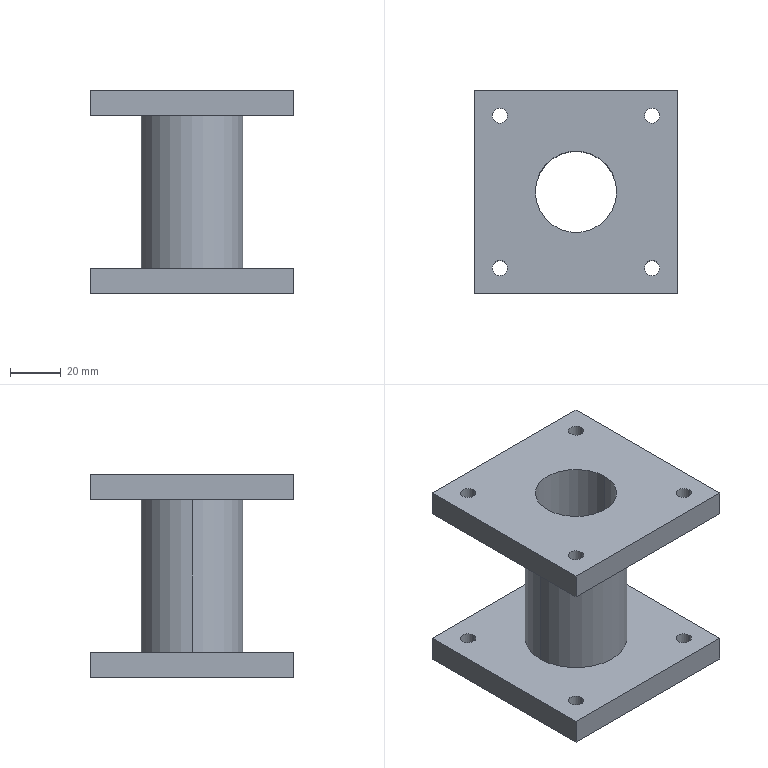Part | STEP file | Square tube | 1 solid | 32 faces | box 80 x 80 x 80 mm | volume 136796 mm3 | cylinder 20 | plane 12 | commonest cylinder face diameters 6 x16 32 x2 40 x2
STEP:
#1=CARTESIAN_POINT('',(33.,-30.,10.));
#2=VERTEX_POINT('',#1);
#3=CARTESIAN_POINT('',(27.,-30.,10.));
#4=VERTEX_POINT('',#3);
#5=CARTESIAN_POINT('',(30.,-30.,10.));
#6=DIRECTION('',(0.,0.,-1.));
#7=DIRECTION('',(-1.,0.,0.));
#8=AXIS2_PLACEMENT_3D('',#5,#6,#7);
#9=CIRCLE('',#8,3.);
#10=EDGE_CURVE('',#2,#4,#9,.T.);
#11=ORIENTED_EDGE('',*,*,#10,.F.);
#12=CARTESIAN_POINT('',(33.,-30.,0.));
#13=VERTEX_POINT('',#12);
#14=CARTESIAN_POINT('',(33.,-30.,10.));
#15=DIRECTION('',(0.,0.,-1.));
#16=VECTOR('',#15,1000.);
#17=LINE('',#14,#16);
#18=EDGE_CURVE('',#2,#13,#17,.T.);
#19=ORIENTED_EDGE('',*,*,#18,.T.);
#20=CARTESIAN_POINT('',(27.,-30.,0.));
#21=VERTEX_POINT('',#20);
#22=CARTESIAN_POINT('',(30.,-30.,0.));
#23=DIRECTION('',(0.,0.,-1.));
#24=DIRECTION('',(-1.,0.,0.));
#25=AXIS2_PLACEMENT_3D('',#22,#23,#24);
#26=CIRCLE('',#25,3.);
#27=EDGE_CURVE('',#13,#21,#26,.T.);
#28=ORIENTED_EDGE('',*,*,#27,.T.);
#29=CARTESIAN_POINT('',(27.,-30.,10.));
#30=DIRECTION('',(0.,0.,-1.));
#31=VECTOR('',#30,1000.);
#32=LINE('',#29,#31);
#33=EDGE_CURVE('',#4,#21,#32,.T.);
#34=ORIENTED_EDGE('',*,*,#33,.F.);
#35=EDGE_LOOP('',(#11,#19,#28,#34));
#36=FACE_OUTER_BOUND('',#35,.T.);
#37=CARTESIAN_POINT('',(30.,-30.,10.));
#38=DIRECTION('',(0.,0.,-1.));
#39=DIRECTION('',(-1.,0.,0.));
#40=AXIS2_PLACEMENT_3D('',#37,#38,#39);
#41=CYLINDRICAL_SURFACE('',#40,3.);
#42=ADVANCED_FACE('',(#36),#41,.F.);
#43=CARTESIAN_POINT('',(33.,30.,10.));
#44=VERTEX_POINT('',#43);
#45=CARTESIAN_POINT('',(27.,30.,10.));
#46=VERTEX_POINT('',#45);
#47=CARTESIAN_POINT('',(30.,30.,10.));
#48=DIRECTION('',(0.,0.,-1.));
#49=DIRECTION('',(-1.,0.,0.));
#50=AXIS2_PLACEMENT_3D('',#47,#48,#49);
#51=CIRCLE('',#50,3.);
#52=EDGE_CURVE('',#44,#46,#51,.T.);
#53=ORIENTED_EDGE('',*,*,#52,.F.);
#54=CARTESIAN_POINT('',(33.,30.,0.));
#55=VERTEX_POINT('',#54);
#56=CARTESIAN_POINT('',(33.,30.,10.));
#57=DIRECTION('',(0.,0.,-1.));
#58=VECTOR('',#57,1000.);
#59=LINE('',#56,#58);
#60=EDGE_CURVE('',#44,#55,#59,.T.);
#61=ORIENTED_EDGE('',*,*,#60,.T.);
#62=CARTESIAN_POINT('',(27.,30.,0.));
#63=VERTEX_POINT('',#62);
#64=CARTESIAN_POINT('',(30.,30.,0.));
#65=DIRECTION('',(0.,0.,-1.));
#66=DIRECTION('',(-1.,0.,0.));
#67=AXIS2_PLACEMENT_3D('',#64,#65,#66);
#68=CIRCLE('',#67,3.);
#69=EDGE_CURVE('',#55,#63,#68,.T.);
#70=ORIENTED_EDGE('',*,*,#69,.T.);
#71=CARTESIAN_POINT('',(27.,30.,10.));
#72=DIRECTION('',(0.,0.,-1.));
#73=VECTOR('',#72,1000.);
#74=LINE('',#71,#73);
#75=EDGE_CURVE('',#46,#63,#74,.T.);
#76=ORIENTED_EDGE('',*,*,#75,.F.);
#77=EDGE_LOOP('',(#53,#61,#70,#76));
#78=FACE_OUTER_BOUND('',#77,.T.);
#79=CARTESIAN_POINT('',(30.,30.,10.));
#80=DIRECTION('',(0.,0.,-1.));
#81=DIRECTION('',(-1.,0.,0.));
#82=AXIS2_PLACEMENT_3D('',#79,#80,#81);
#83=CYLINDRICAL_SURFACE('',#82,3.);
#84=ADVANCED_FACE('',(#78),#83,.F.);
#85=CARTESIAN_POINT('',(-27.,30.,10.));
#86=VERTEX_POINT('',#85);
#87=CARTESIAN_POINT('',(-33.,30.,10.));
#88=VERTEX_POINT('',#87);
#89=CARTESIAN_POINT('',(-30.,30.,10.));
#90=DIRECTION('',(0.,0.,-1.));
#91=DIRECTION('',(-1.,0.,0.));
#92=AXIS2_PLACEMENT_3D('',#89,#90,#91);
#93=CIRCLE('',#92,3.);
#94=EDGE_CURVE('',#86,#88,#93,.T.);
#95=ORIENTED_EDGE('',*,*,#94,.F.);
#96=CARTESIAN_POINT('',(-27.,30.,0.));
#97=VERTEX_POINT('',#96);
#98=CARTESIAN_POINT('',(-27.,30.,10.));
#99=DIRECTION('',(0.,0.,-1.));
#100=VECTOR('',#99,1000.);
#101=LINE('',#98,#100);
#102=EDGE_CURVE('',#86,#97,#101,.T.);
#103=ORIENTED_EDGE('',*,*,#102,.T.);
#104=CARTESIAN_POINT('',(-33.,30.,0.));
#105=VERTEX_POINT('',#104);
#106=CARTESIAN_POINT('',(-30.,30.,0.));
#107=DIRECTION('',(0.,0.,-1.));
#108=DIRECTION('',(-1.,0.,0.));
#109=AXIS2_PLACEMENT_3D('',#106,#107,#108);
#110=CIRCLE('',#109,3.);
#111=EDGE_CURVE('',#97,#105,#110,.T.);
#112=ORIENTED_EDGE('',*,*,#111,.T.);
#113=CARTESIAN_POINT('',(-33.,30.,10.));
#114=DIRECTION('',(0.,0.,-1.));
#115=VECTOR('',#114,1000.);
#116=LINE('',#113,#115);
#117=EDGE_CURVE('',#88,#105,#116,.T.);
#118=ORIENTED_EDGE('',*,*,#117,.F.);
#119=EDGE_LOOP('',(#95,#103,#112,#118));
#120=FACE_OUTER_BOUND('',#119,.T.);
#121=CARTESIAN_POINT('',(-30.,30.,10.));
#122=DIRECTION('',(0.,0.,-1.));
#123=DIRECTION('',(-1.,0.,0.));
#124=AXIS2_PLACEMENT_3D('',#121,#122,#123);
#125=CYLINDRICAL_SURFACE('',#124,3.);
#126=ADVANCED_FACE('',(#120),#125,.F.);
#127=CARTESIAN_POINT('',(-27.,-30.,10.));
#128=VERTEX_POINT('',#127);
#129=CARTESIAN_POINT('',(-33.,-30.,10.));
#130=VERTEX_POINT('',#129);
#131=CARTESIAN_POINT('',(-30.,-30.,10.));
#132=DIRECTION('',(0.,0.,-1.));
#133=DIRECTION('',(-1.,0.,0.));
#134=AXIS2_PLACEMENT_3D('',#131,#132,#133);
#135=CIRCLE('',#134,3.);
#136=EDGE_CURVE('',#128,#130,#135,.T.);
#137=ORIENTED_EDGE('',*,*,#136,.F.);
#138=CARTESIAN_POINT('',(-27.,-30.,0.));
#139=VERTEX_POINT('',#138);
#140=CARTESIAN_POINT('',(-27.,-30.,10.));
#141=DIRECTION('',(0.,0.,-1.));
#142=VECTOR('',#141,1000.);
#143=LINE('',#140,#142);
#144=EDGE_CURVE('',#128,#139,#143,.T.);
#145=ORIENTED_EDGE('',*,*,#144,.T.);
#146=CARTESIAN_POINT('',(-33.,-30.,0.));
#147=VERTEX_POINT('',#146);
#148=CARTESIAN_POINT('',(-30.,-30.,0.));
#149=DIRECTION('',(0.,0.,-1.));
#150=DIRECTION('',(-1.,0.,0.));
#151=AXIS2_PLACEMENT_3D('',#148,#149,#150);
#152=CIRCLE('',#151,3.);
#153=EDGE_CURVE('',#139,#147,#152,.T.);
#154=ORIENTED_EDGE('',*,*,#153,.T.);
#155=CARTESIAN_POINT('',(-33.,-30.,10.));
#156=DIRECTION('',(0.,0.,-1.));
#157=VECTOR('',#156,1000.);
#158=LINE('',#155,#157);
#159=EDGE_CURVE('',#130,#147,#158,.T.);
#160=ORIENTED_EDGE('',*,*,#159,.F.);
#161=EDGE_LOOP('',(#137,#145,#154,#160));
#162=FACE_OUTER_BOUND('',#161,.T.);
#163=CARTESIAN_POINT('',(-30.,-30.,10.));
#164=DIRECTION('',(0.,0.,-1.));
#165=DIRECTION('',(-1.,0.,0.));
#166=AXIS2_PLACEMENT_3D('',#163,#164,#165);
#167=CYLINDRICAL_SURFACE('',#166,3.);
#168=ADVANCED_FACE('',(#162),#167,.F.);
#169=CARTESIAN_POINT('',(16.,0.,80.));
#170=VERTEX_POINT('',#169);
#171=CARTESIAN_POINT('',(-16.,0.,80.));
#172=VERTEX_POINT('',#171);
#173=CARTESIAN_POINT('',(0.,0.,80.));
#174=DIRECTION('',(0.,0.,-1.));
#175=DIRECTION('',(-1.,0.,0.));
#176=AXIS2_PLACEMENT_3D('',#173,#174,#175);
#177=CIRCLE('',#176,16.);
#178=EDGE_CURVE('',#170,#172,#177,.T.);
#179=ORIENTED_EDGE('',*,*,#178,.F.);
#180=CARTESIAN_POINT('',(16.,0.,0.));
#181=VERTEX_POINT('',#180);
#182=CARTESIAN_POINT('',(16.,0.,70.));
#183=DIRECTION('',(0.,0.,-1.));
#184=VECTOR('',#183,1000.);
#185=LINE('',#182,#184);
#186=EDGE_CURVE('',#170,#181,#185,.T.);
#187=ORIENTED_EDGE('',*,*,#186,.T.);
#188=CARTESIAN_POINT('',(-16.,0.,0.));
#189=VERTEX_POINT('',#188);
#190=CARTESIAN_POINT('',(0.,0.,0.));
#191=DIRECTION('',(0.,0.,-1.));
#192=DIRECTION('',(-1.,0.,0.));
#193=AXIS2_PLACEMENT_3D('',#190,#191,#192);
#194=CIRCLE('',#193,16.);
#195=EDGE_CURVE('',#181,#189,#194,.T.);
#196=ORIENTED_EDGE('',*,*,#195,.T.);
#197=CARTESIAN_POINT('',(-16.,0.,70.));
#198=DIRECTION('',(0.,0.,-1.));
#199=VECTOR('',#198,1000.);
#200=LINE('',#197,#199);
#201=EDGE_CURVE('',#172,#189,#200,.T.);
#202=ORIENTED_EDGE('',*,*,#201,.F.);
#203=EDGE_LOOP('',(#179,#187,#196,#202));
#204=FACE_OUTER_BOUND('',#203,.T.);
#205=CARTESIAN_POINT('',(0.,0.,70.));
#206=DIRECTION('',(0.,0.,-1.));
#207=DIRECTION('',(-1.,0.,0.));
#208=AXIS2_PLACEMENT_3D('',#205,#206,#207);
#209=CYLINDRICAL_SURFACE('',#208,16.);
#210=ADVANCED_FACE('',(#204),#209,.F.);
#211=CARTESIAN_POINT('',(-20.,0.,70.));
#212=VERTEX_POINT('',#211);
#213=CARTESIAN_POINT('',(20.,0.,70.));
#214=VERTEX_POINT('',#213);
#215=CARTESIAN_POINT('',(0.,0.,70.));
#216=DIRECTION('',(0.,0.,-1.));
#217=DIRECTION('',(-1.,0.,0.));
#218=AXIS2_PLACEMENT_3D('',#215,#216,#217);
#219=CIRCLE('',#218,20.);
#220=EDGE_CURVE('',#212,#214,#219,.T.);
#221=ORIENTED_EDGE('',*,*,#220,.T.);
#222=CARTESIAN_POINT('',(20.,0.,10.));
#223=VERTEX_POINT('',#222);
#224=CARTESIAN_POINT('',(20.,0.,70.));
#225=DIRECTION('',(0.,0.,-1.));
#226=VECTOR('',#225,1000.);
#227=LINE('',#224,#226);
#228=EDGE_CURVE('',#214,#223,#227,.T.);
#229=ORIENTED_EDGE('',*,*,#228,.T.);
#230=CARTESIAN_POINT('',(-20.,0.,10.));
#231=VERTEX_POINT('',#230);
#232=CARTESIAN_POINT('',(0.,0.,10.));
#233=DIRECTION('',(0.,0.,-1.));
#234=DIRECTION('',(-1.,0.,0.));
#235=AXIS2_PLACEMENT_3D('',#232,#233,#234);
#236=CIRCLE('',#235,20.);
#237=EDGE_CURVE('',#231,#223,#236,.T.);
#238=ORIENTED_EDGE('',*,*,#237,.F.);
#239=CARTESIAN_POINT('',(-20.,0.,70.));
#240=DIRECTION('',(0.,0.,-1.));
#241=VECTOR('',#240,1000.);
#242=LINE('',#239,#241);
#243=EDGE_CURVE('',#212,#231,#242,.T.);
#244=ORIENTED_EDGE('',*,*,#243,.F.);
#245=EDGE_LOOP('',(#221,#229,#238,#244));
#246=FACE_OUTER_BOUND('',#245,.T.);
#247=CARTESIAN_POINT('',(0.,0.,70.));
#248=DIRECTION('',(0.,0.,-1.));
#249=DIRECTION('',(-1.,0.,0.));
#250=AXIS2_PLACEMENT_3D('',#247,#248,#249);
#251=CYLINDRICAL_SURFACE('',#250,20.);
#252=ADVANCED_FACE('',(#246),#251,.T.);
#253=CARTESIAN_POINT('',(-27.,-30.,80.));
#254=VERTEX_POINT('',#253);
#255=CARTESIAN_POINT('',(-33.,-30.,80.));
#256=VERTEX_POINT('',#255);
#257=CARTESIAN_POINT('',(-30.,-30.,80.));
#258=DIRECTION('',(0.,0.,-1.));
#259=DIRECTION('',(-1.,0.,0.));
#260=AXIS2_PLACEMENT_3D('',#257,#258,#259);
#261=CIRCLE('',#260,3.);
#262=EDGE_CURVE('',#254,#256,#261,.T.);
#263=ORIENTED_EDGE('',*,*,#262,.F.);
#264=CARTESIAN_POINT('',(-27.,-30.,70.));
#265=VERTEX_POINT('',#264);
#266=CARTESIAN_POINT('',(-27.,-30.,80.));
#267=DIRECTION('',(0.,0.,-1.));
#268=VECTOR('',#267,1000.);
#269=LINE('',#266,#268);
#270=EDGE_CURVE('',#254,#265,#269,.T.);
#271=ORIENTED_EDGE('',*,*,#270,.T.);
#272=CARTESIAN_POINT('',(-33.,-30.,70.));
#273=VERTEX_POINT('',#272);
#274=CARTESIAN_POINT('',(-30.,-30.,70.));
#275=DIRECTION('',(0.,0.,1.));
#276=DIRECTION('',(-1.,0.,0.));
#277=AXIS2_PLACEMENT_3D('',#274,#275,#276);
#278=CIRCLE('',#277,3.);
#279=EDGE_CURVE('',#273,#265,#278,.T.);
#280=ORIENTED_EDGE('',*,*,#279,.F.);
#281=CARTESIAN_POINT('',(-33.,-30.,80.));
#282=DIRECTION('',(0.,0.,-1.));
#283=VECTOR('',#282,1000.);
#284=LINE('',#281,#283);
#285=EDGE_CURVE('',#256,#273,#284,.T.);
#286=ORIENTED_EDGE('',*,*,#285,.F.);
#287=EDGE_LOOP('',(#263,#271,#280,#286));
#288=FACE_OUTER_BOUND('',#287,.T.);
#289=CARTESIAN_POINT('',(-30.,-30.,80.));
#290=DIRECTION('',(0.,0.,-1.));
#291=DIRECTION('',(-1.,0.,0.));
#292=AXIS2_PLACEMENT_3D('',#289,#290,#291);
#293=CYLINDRICAL_SURFACE('',#292,3.);
#294=ADVANCED_FACE('',(#288),#293,.F.);
#295=CARTESIAN_POINT('',(33.,30.,80.));
#296=VERTEX_POINT('',#295);
#297=CARTESIAN_POINT('',(27.,30.,80.));
#298=VERTEX_POINT('',#297);
#299=CARTESIAN_POINT('',(30.,30.,80.));
#300=DIRECTION('',(0.,0.,-1.));
#301=DIRECTION('',(-1.,0.,0.));
#302=AXIS2_PLACEMENT_3D('',#299,#300,#301);
#303=CIRCLE('',#302,3.);
#304=EDGE_CURVE('',#296,#298,#303,.T.);
#305=ORIENTED_EDGE('',*,*,#304,.F.);
#306=CARTESIAN_POINT('',(33.,30.,70.));
#307=VERTEX_POINT('',#306);
#308=CARTESIAN_POINT('',(33.,30.,80.));
#309=DIRECTION('',(0.,0.,-1.));
#310=VECTOR('',#309,1000.);
#311=LINE('',#308,#310);
#312=EDGE_CURVE('',#296,#307,#311,.T.);
#313=ORIENTED_EDGE('',*,*,#312,.T.);
#314=CARTESIAN_POINT('',(27.,30.,70.));
#315=VERTEX_POINT('',#314);
#316=CARTESIAN_POINT('',(30.,30.,70.));
#317=DIRECTION('',(0.,0.,1.));
#318=DIRECTION('',(-1.,0.,0.));
#319=AXIS2_PLACEMENT_3D('',#316,#317,#318);
#320=CIRCLE('',#319,3.);
#321=EDGE_CURVE('',#315,#307,#320,.T.);
#322=ORIENTED_EDGE('',*,*,#321,.F.);
#323=CARTESIAN_POINT('',(27.,30.,80.));
#324=DIRECTION('',(0.,0.,-1.));
#325=VECTOR('',#324,1000.);
#326=LINE('',#323,#325);
#327=EDGE_CURVE('',#298,#315,#326,.T.);
#328=ORIENTED_EDGE('',*,*,#327,.F.);
#329=EDGE_LOOP('',(#305,#313,#322,#328));
#330=FACE_OUTER_BOUND('',#329,.T.);
#331=CARTESIAN_POINT('',(30.,30.,80.));
#332=DIRECTION('',(0.,0.,-1.));
#333=DIRECTION('',(-1.,0.,0.));
#334=AXIS2_PLACEMENT_3D('',#331,#332,#333);
#335=CYLINDRICAL_SURFACE('',#334,3.);
#336=ADVANCED_FACE('',(#330),#335,.F.);
#337=CARTESIAN_POINT('',(-27.,30.,80.));
#338=VERTEX_POINT('',#337);
#339=CARTESIAN_POINT('',(-33.,30.,80.));
#340=VERTEX_POINT('',#339);
#341=CARTESIAN_POINT('',(-30.,30.,80.));
#342=DIRECTION('',(0.,0.,-1.));
#343=DIRECTION('',(-1.,0.,0.));
#344=AXIS2_PLACEMENT_3D('',#341,#342,#343);
#345=CIRCLE('',#344,3.);
#346=EDGE_CURVE('',#338,#340,#345,.T.);
#347=ORIENTED_EDGE('',*,*,#346,.F.);
#348=CARTESIAN_POINT('',(-27.,30.,70.));
#349=VERTEX_POINT('',#348);
#350=CARTESIAN_POINT('',(-27.,30.,80.));
#351=DIRECTION('',(0.,0.,-1.));
#352=VECTOR('',#351,1000.);
#353=LINE('',#350,#352);
#354=EDGE_CURVE('',#338,#349,#353,.T.);
#355=ORIENTED_EDGE('',*,*,#354,.T.);
#356=CARTESIAN_POINT('',(-33.,30.,70.));
#357=VERTEX_POINT('',#356);
#358=CARTESIAN_POINT('',(-30.,30.,70.));
#359=DIRECTION('',(0.,0.,1.));
#360=DIRECTION('',(-1.,0.,0.));
#361=AXIS2_PLACEMENT_3D('',#358,#359,#360);
#362=CIRCLE('',#361,3.);
#363=EDGE_CURVE('',#357,#349,#362,.T.);
#364=ORIENTED_EDGE('',*,*,#363,.F.);
#365=CARTESIAN_POINT('',(-33.,30.,80.));
#366=DIRECTION('',(0.,0.,-1.));
#367=VECTOR('',#366,1000.);
#368=LINE('',#365,#367);
#369=EDGE_CURVE('',#340,#357,#368,.T.);
#370=ORIENTED_EDGE('',*,*,#369,.F.);
#371=EDGE_LOOP('',(#347,#355,#364,#370));
#372=FACE_OUTER_BOUND('',#371,.T.);
#373=CARTESIAN_POINT('',(-30.,30.,80.));
#374=DIRECTION('',(0.,0.,-1.));
#375=DIRECTION('',(-1.,0.,0.));
#376=AXIS2_PLACEMENT_3D('',#373,#374,#375);
#377=CYLINDRICAL_SURFACE('',#376,3.);
#378=ADVANCED_FACE('',(#372),#377,.F.);
#379=CARTESIAN_POINT('',(33.,-30.,80.));
#380=VERTEX_POINT('',#379);
#381=CARTESIAN_POINT('',(27.,-30.,80.));
#382=VERTEX_POINT('',#381);
#383=CARTESIAN_POINT('',(30.,-30.,80.));
#384=DIRECTION('',(0.,0.,-1.));
#385=DIRECTION('',(-1.,0.,0.));
#386=AXIS2_PLACEMENT_3D('',#383,#384,#385);
#387=CIRCLE('',#386,3.);
#388=EDGE_CURVE('',#380,#382,#387,.T.);
#389=ORIENTED_EDGE('',*,*,#388,.F.);
#390=CARTESIAN_POINT('',(33.,-30.,70.));
#391=VERTEX_POINT('',#390);
#392=CARTESIAN_POINT('',(33.,-30.,80.));
#393=DIRECTION('',(0.,0.,-1.));
#394=VECTOR('',#393,1000.);
#395=LINE('',#392,#394);
#396=EDGE_CURVE('',#380,#391,#395,.T.);
#397=ORIENTED_EDGE('',*,*,#396,.T.);
#398=CARTESIAN_POINT('',(27.,-30.,70.));
#399=VERTEX_POINT('',#398);
#400=CARTESIAN_POINT('',(30.,-30.,70.));
#401=DIRECTION('',(0.,0.,1.));
#402=DIRECTION('',(-1.,0.,0.));
#403=AXIS2_PLACEMENT_3D('',#400,#401,#402);
#404=CIRCLE('',#403,3.);
#405=EDGE_CURVE('',#399,#391,#404,.T.);
#406=ORIENTED_EDGE('',*,*,#405,.F.);
#407=CARTESIAN_POINT('',(27.,-30.,80.));
#408=DIRECTION('',(0.,0.,-1.));
#409=VECTOR('',#408,1000.);
#410=LINE('',#407,#409);
#411=EDGE_CURVE('',#382,#399,#410,.T.);
#412=ORIENTED_EDGE('',*,*,#411,.F.);
#413=EDGE_LOOP('',(#389,#397,#406,#412));
#414=FACE_OUTER_BOUND('',#413,.T.);
#415=CARTESIAN_POINT('',(30.,-30.,80.));
#416=DIRECTION('',(0.,0.,-1.));
#417=DIRECTION('',(-1.,0.,0.));
#418=AXIS2_PLACEMENT_3D('',#415,#416,#417);
#419=CYLINDRICAL_SURFACE('',#418,3.);
#420=ADVANCED_FACE('',(#414),#419,.F.);
#421=CARTESIAN_POINT('',(30.,-30.,0.));
#422=DIRECTION('',(0.,0.,-1.));
#423=DIRECTION('',(-1.,0.,0.));
#424=AXIS2_PLACEMENT_3D('',#421,#422,#423);
#425=CIRCLE('',#424,3.);
#426=EDGE_CURVE('',#21,#13,#425,.T.);
#427=ORIENTED_EDGE('',*,*,#426,.F.);
#428=ORIENTED_EDGE('',*,*,#27,.F.);
#429=EDGE_LOOP('',(#427,#428));
#430=FACE_BOUND('',#429,.T.);
#431=CARTESIAN_POINT('',(30.,30.,0.));
#432=DIRECTION('',(0.,0.,-1.));
#433=DIRECTION('',(-1.,0.,0.));
#434=AXIS2_PLACEMENT_3D('',#431,#432,#433);
#435=CIRCLE('',#434,3.);
#436=EDGE_CURVE('',#63,#55,#435,.T.);
#437=ORIENTED_EDGE('',*,*,#436,.F.);
#438=ORIENTED_EDGE('',*,*,#69,.F.);
#439=EDGE_LOOP('',(#437,#438));
#440=FACE_BOUND('',#439,.T.);
#441=CARTESIAN_POINT('',(40.,40.,0.));
#442=VERTEX_POINT('',#441);
#443=CARTESIAN_POINT('',(-40.,40.,0.));
#444=VERTEX_POINT('',#443);
#445=CARTESIAN_POINT('',(-40.,40.,0.));
#446=DIRECTION('',(-1.,0.,0.));
#447=VECTOR('',#446,1000.);
#448=LINE('',#445,#447);
#449=EDGE_CURVE('',#442,#444,#448,.T.);
#450=ORIENTED_EDGE('',*,*,#449,.F.);
#451=CARTESIAN_POINT('',(40.,-40.,0.));
#452=VERTEX_POINT('',#451);
#453=CARTESIAN_POINT('',(40.,-40.,0.));
#454=DIRECTION('',(0.,1.,0.));
#455=VECTOR('',#454,1000.);
#456=LINE('',#453,#455);
#457=EDGE_CURVE('',#452,#442,#456,.T.);
#458=ORIENTED_EDGE('',*,*,#457,.F.);
#459=CARTESIAN_POINT('',(-40.,-40.,0.));
#460=VERTEX_POINT('',#459);
#461=CARTESIAN_POINT('',(-40.,-40.,0.));
#462=DIRECTION('',(1.,0.,0.));
#463=VECTOR('',#462,1000.);
#464=LINE('',#461,#463);
#465=EDGE_CURVE('',#460,#452,#464,.T.);
#466=ORIENTED_EDGE('',*,*,#465,.F.);
#467=CARTESIAN_POINT('',(-40.,-40.,0.));
#468=DIRECTION('',(0.,-1.,0.));
#469=VECTOR('',#468,1000.);
#470=LINE('',#467,#469);
#471=EDGE_CURVE('',#444,#460,#470,.T.);
#472=ORIENTED_EDGE('',*,*,#471,.F.);
#473=EDGE_LOOP('',(#450,#458,#466,#472));
#474=FACE_OUTER_BOUND('',#473,.T.);
#475=CARTESIAN_POINT('',(-30.,30.,0.));
#476=DIRECTION('',(0.,0.,-1.));
#477=DIRECTION('',(-1.,0.,0.));
#478=AXIS2_PLACEMENT_3D('',#475,#476,#477);
#479=CIRCLE('',#478,3.);
#480=EDGE_CURVE('',#105,#97,#479,.T.);
#481=ORIENTED_EDGE('',*,*,#480,.F.);
#482=ORIENTED_EDGE('',*,*,#111,.F.);
#483=EDGE_LOOP('',(#481,#482));
#484=FACE_BOUND('',#483,.T.);
#485=CARTESIAN_POINT('',(-30.,-30.,0.));
#486=DIRECTION('',(0.,0.,-1.));
#487=DIRECTION('',(-1.,0.,0.));
#488=AXIS2_PLACEMENT_3D('',#485,#486,#487);
#489=CIRCLE('',#488,3.);
#490=EDGE_CURVE('',#147,#139,#489,.T.);
#491=ORIENTED_EDGE('',*,*,#490,.F.);
#492=ORIENTED_EDGE('',*,*,#153,.F.);
#493=EDGE_LOOP('',(#491,#492));
#494=FACE_BOUND('',#493,.T.);
#495=CARTESIAN_POINT('',(0.,0.,0.));
#496=DIRECTION('',(0.,0.,-1.));
#497=DIRECTION('',(-1.,0.,0.));
#498=AXIS2_PLACEMENT_3D('',#495,#496,#497);
#499=CIRCLE('',#498,16.);
#500=EDGE_CURVE('',#189,#181,#499,.T.);
#501=ORIENTED_EDGE('',*,*,#500,.F.);
#502=ORIENTED_EDGE('',*,*,#195,.F.);
#503=EDGE_LOOP('',(#501,#502));
#504=FACE_BOUND('',#503,.T.);
#505=CARTESIAN_POINT('',(-40.,-40.,0.));
#506=DIRECTION('',(0.,0.,1.));
#507=DIRECTION('',(1.,0.,0.));
#508=AXIS2_PLACEMENT_3D('',#505,#506,#507);
#509=PLANE('',#508);
#510=ADVANCED_FACE('',(#430,#440,#474,#484,#494,#504),#509,.F.);
#511=ORIENTED_EDGE('',*,*,#18,.F.);
#512=CARTESIAN_POINT('',(30.,-30.,10.));
#513=DIRECTION('',(0.,0.,-1.));
#514=DIRECTION('',(-1.,0.,0.));
#515=AXIS2_PLACEMENT_3D('',#512,#513,#514);
#516=CIRCLE('',#515,3.);
#517=EDGE_CURVE('',#4,#2,#516,.T.);
#518=ORIENTED_EDGE('',*,*,#517,.F.);
#519=ORIENTED_EDGE('',*,*,#33,.T.);
#520=ORIENTED_EDGE('',*,*,#426,.T.);
#521=EDGE_LOOP('',(#511,#518,#519,#520));
#522=FACE_OUTER_BOUND('',#521,.T.);
#523=CARTESIAN_POINT('',(30.,-30.,10.));
#524=DIRECTION('',(0.,0.,-1.));
#525=DIRECTION('',(-1.,0.,0.));
#526=AXIS2_PLACEMENT_3D('',#523,#524,#525);
#527=CYLINDRICAL_SURFACE('',#526,3.);
#528=ADVANCED_FACE('',(#522),#527,.F.);
#529=ORIENTED_EDGE('',*,*,#60,.F.);
#530=CARTESIAN_POINT('',(30.,30.,10.));
#531=DIRECTION('',(0.,0.,-1.));
#532=DIRECTION('',(-1.,0.,0.));
#533=AXIS2_PLACEMENT_3D('',#530,#531,#532);
#534=CIRCLE('',#533,3.);
#535=EDGE_CURVE('',#46,#44,#534,.T.);
#536=ORIENTED_EDGE('',*,*,#535,.F.);
#537=ORIENTED_EDGE('',*,*,#75,.T.);
#538=ORIENTED_EDGE('',*,*,#436,.T.);
#539=EDGE_LOOP('',(#529,#536,#537,#538));
#540=FACE_OUTER_BOUND('',#539,.T.);
#541=CARTESIAN_POINT('',(30.,30.,10.));
#542=DIRECTION('',(0.,0.,-1.));
#543=DIRECTION('',(-1.,0.,0.));
#544=AXIS2_PLACEMENT_3D('',#541,#542,#543);
#545=CYLINDRICAL_SURFACE('',#544,3.);
#546=ADVANCED_FACE('',(#540),#545,.F.);
#547=CARTESIAN_POINT('',(-40.,-40.,10.));
#548=VERTEX_POINT('',#547);
#549=CARTESIAN_POINT('',(-40.,-40.,10.));
#550=DIRECTION('',(0.,0.,-1.));
#551=VECTOR('',#550,1000.);
#552=LINE('',#549,#551);
#553=EDGE_CURVE('',#548,#460,#552,.T.);
#554=ORIENTED_EDGE('',*,*,#553,.F.);
#555=CARTESIAN_POINT('',(-40.,40.,10.));
#556=VERTEX_POINT('',#555);
#557=CARTESIAN_POINT('',(-40.,40.,10.));
#558=DIRECTION('',(0.,-1.,0.));
#559=VECTOR('',#558,1000.);
#560=LINE('',#557,#559);
#561=EDGE_CURVE('',#556,#548,#560,.T.);
#562=ORIENTED_EDGE('',*,*,#561,.F.);
#563=CARTESIAN_POINT('',(-40.,40.,10.));
#564=DIRECTION('',(0.,0.,1.));
#565=VECTOR('',#564,1000.);
#566=LINE('',#563,#565);
#567=EDGE_CURVE('',#444,#556,#566,.T.);
#568=ORIENTED_EDGE('',*,*,#567,.F.);
#569=ORIENTED_EDGE('',*,*,#471,.T.);
#570=EDGE_LOOP('',(#554,#562,#568,#569));
#571=FACE_OUTER_BOUND('',#570,.T.);
#572=CARTESIAN_POINT('',(-40.,40.,10.));
#573=DIRECTION('',(1.,0.,0.));
#574=DIRECTION('',(0.,1.,0.));
#575=AXIS2_PLACEMENT_3D('',#572,#573,#574);
#576=PLANE('',#575);
#577=ADVANCED_FACE('',(#571),#576,.F.);
#578=ORIENTED_EDGE('',*,*,#567,.T.);
#579=CARTESIAN_POINT('',(40.,40.,10.));
#580=VERTEX_POINT('',#579);
#581=CARTESIAN_POINT('',(-40.,40.,10.));
#582=DIRECTION('',(-1.,0.,0.));
#583=VECTOR('',#582,1000.);
#584=LINE('',#581,#583);
#585=EDGE_CURVE('',#580,#556,#584,.T.);
#586=ORIENTED_EDGE('',*,*,#585,.F.);
#587=CARTESIAN_POINT('',(40.,40.,10.));
#588=DIRECTION('',(0.,0.,1.));
#589=VECTOR('',#588,1000.);
#590=LINE('',#587,#589);
#591=EDGE_CURVE('',#442,#580,#590,.T.);
#592=ORIENTED_EDGE('',*,*,#591,.F.);
#593=ORIENTED_EDGE('',*,*,#449,.T.);
#594=EDGE_LOOP('',(#578,#586,#592,#593));
#595=FACE_OUTER_BOUND('',#594,.T.);
#596=CARTESIAN_POINT('',(-40.,40.,10.));
#597=DIRECTION('',(0.,-1.,0.));
#598=DIRECTION('',(1.,0.,0.));
#599=AXIS2_PLACEMENT_3D('',#596,#597,#598);
#600=PLANE('',#599);
#601=ADVANCED_FACE('',(#595),#600,.F.);
#602=ORIENTED_EDGE('',*,*,#591,.T.);
#603=CARTESIAN_POINT('',(40.,-40.,10.));
#604=VERTEX_POINT('',#603);
#605=CARTESIAN_POINT('',(40.,40.,10.));
#606=DIRECTION('',(0.,1.,0.));
#607=VECTOR('',#606,1000.);
#608=LINE('',#605,#607);
#609=EDGE_CURVE('',#604,#580,#608,.T.);
#610=ORIENTED_EDGE('',*,*,#609,.F.);
#611=CARTESIAN_POINT('',(40.,-40.,10.));
#612=DIRECTION('',(0.,0.,1.));
#613=VECTOR('',#612,1000.);
#614=LINE('',#611,#613);
#615=EDGE_CURVE('',#452,#604,#614,.T.);
#616=ORIENTED_EDGE('',*,*,#615,.F.);
#617=ORIENTED_EDGE('',*,*,#457,.T.);
#618=EDGE_LOOP('',(#602,#610,#616,#617));
#619=FACE_OUTER_BOUND('',#618,.T.);
#620=CARTESIAN_POINT('',(40.,40.,10.));
#621=DIRECTION('',(-1.,0.,0.));
#622=DIRECTION('',(0.,-1.,0.));
#623=AXIS2_PLACEMENT_3D('',#620,#621,#622);
#624=PLANE('',#623);
#625=ADVANCED_FACE('',(#619),#624,.F.);
#626=ORIENTED_EDGE('',*,*,#615,.T.);
#627=CARTESIAN_POINT('',(-40.,-40.,10.));
#628=DIRECTION('',(1.,0.,0.));
#629=VECTOR('',#628,1000.);
#630=LINE('',#627,#629);
#631=EDGE_CURVE('',#548,#604,#630,.T.);
#632=ORIENTED_EDGE('',*,*,#631,.F.);
#633=ORIENTED_EDGE('',*,*,#553,.T.);
#634=ORIENTED_EDGE('',*,*,#465,.T.);
#635=EDGE_LOOP('',(#626,#632,#633,#634));
#636=FACE_OUTER_BOUND('',#635,.T.);
#637=CARTESIAN_POINT('',(-40.,-40.,10.));
#638=DIRECTION('',(0.,1.,0.));
#639=DIRECTION('',(-1.,0.,0.));
#640=AXIS2_PLACEMENT_3D('',#637,#638,#639);
#641=PLANE('',#640);
#642=ADVANCED_FACE('',(#636),#641,.F.);
#643=ORIENTED_EDGE('',*,*,#102,.F.);
#644=CARTESIAN_POINT('',(-30.,30.,10.));
#645=DIRECTION('',(0.,0.,-1.));
#646=DIRECTION('',(-1.,0.,0.));
#647=AXIS2_PLACEMENT_3D('',#644,#645,#646);
#648=CIRCLE('',#647,3.);
#649=EDGE_CURVE('',#88,#86,#648,.T.);
#650=ORIENTED_EDGE('',*,*,#649,.F.);
#651=ORIENTED_EDGE('',*,*,#117,.T.);
#652=ORIENTED_EDGE('',*,*,#480,.T.);
#653=EDGE_LOOP('',(#643,#650,#651,#652));
#654=FACE_OUTER_BOUND('',#653,.T.);
#655=CARTESIAN_POINT('',(-30.,30.,10.));
#656=DIRECTION('',(0.,0.,-1.));
#657=DIRECTION('',(-1.,0.,0.));
#658=AXIS2_PLACEMENT_3D('',#655,#656,#657);
#659=CYLINDRICAL_SURFACE('',#658,3.);
#660=ADVANCED_FACE('',(#654),#659,.F.);
#661=ORIENTED_EDGE('',*,*,#144,.F.);
#662=CARTESIAN_POINT('',(-30.,-30.,10.));
#663=DIRECTION('',(0.,0.,-1.));
#664=DIRECTION('',(-1.,0.,0.));
#665=AXIS2_PLACEMENT_3D('',#662,#663,#664);
#666=CIRCLE('',#665,3.);
#667=EDGE_CURVE('',#130,#128,#666,.T.);
#668=ORIENTED_EDGE('',*,*,#667,.F.);
#669=ORIENTED_EDGE('',*,*,#159,.T.);
#670=ORIENTED_EDGE('',*,*,#490,.T.);
#671=EDGE_LOOP('',(#661,#668,#669,#670));
#672=FACE_OUTER_BOUND('',#671,.T.);
#673=CARTESIAN_POINT('',(-30.,-30.,10.));
#674=DIRECTION('',(0.,0.,-1.));
#675=DIRECTION('',(-1.,0.,0.));
#676=AXIS2_PLACEMENT_3D('',#673,#674,#675);
#677=CYLINDRICAL_SURFACE('',#676,3.);
#678=ADVANCED_FACE('',(#672),#677,.F.);
#679=ORIENTED_EDGE('',*,*,#186,.F.);
#680=CARTESIAN_POINT('',(0.,0.,80.));
#681=DIRECTION('',(0.,0.,-1.));
#682=DIRECTION('',(-1.,0.,0.));
#683=AXIS2_PLACEMENT_3D('',#680,#681,#682);
#684=CIRCLE('',#683,16.);
#685=EDGE_CURVE('',#172,#170,#684,.T.);
#686=ORIENTED_EDGE('',*,*,#685,.F.);
#687=ORIENTED_EDGE('',*,*,#201,.T.);
#688=ORIENTED_EDGE('',*,*,#500,.T.);
#689=EDGE_LOOP('',(#679,#686,#687,#688));
#690=FACE_OUTER_BOUND('',#689,.T.);
#691=CARTESIAN_POINT('',(0.,0.,70.));
#692=DIRECTION('',(0.,0.,-1.));
#693=DIRECTION('',(-1.,0.,0.));
#694=AXIS2_PLACEMENT_3D('',#691,#692,#693);
#695=CYLINDRICAL_SURFACE('',#694,16.);
#696=ADVANCED_FACE('',(#690),#695,.F.);
#697=ORIENTED_EDGE('',*,*,#237,.T.);
#698=CARTESIAN_POINT('',(0.,0.,10.));
#699=DIRECTION('',(0.,0.,-1.));
#700=DIRECTION('',(-1.,0.,0.));
#701=AXIS2_PLACEMENT_3D('',#698,#699,#700);
#702=CIRCLE('',#701,20.);
#703=EDGE_CURVE('',#223,#231,#702,.T.);
#704=ORIENTED_EDGE('',*,*,#703,.T.);
#705=EDGE_LOOP('',(#697,#704));
#706=FACE_BOUND('',#705,.T.);
#707=ORIENTED_EDGE('',*,*,#517,.T.);
#708=ORIENTED_EDGE('',*,*,#10,.T.);
#709=EDGE_LOOP('',(#707,#708));
#710=FACE_BOUND('',#709,.T.);
#711=ORIENTED_EDGE('',*,*,#535,.T.);
#712=ORIENTED_EDGE('',*,*,#52,.T.);
#713=EDGE_LOOP('',(#711,#712));
#714=FACE_BOUND('',#713,.T.);
#715=ORIENTED_EDGE('',*,*,#609,.T.);
#716=ORIENTED_EDGE('',*,*,#585,.T.);
#717=ORIENTED_EDGE('',*,*,#561,.T.);
#718=ORIENTED_EDGE('',*,*,#631,.T.);
#719=EDGE_LOOP('',(#715,#716,#717,#718));
#720=FACE_OUTER_BOUND('',#719,.T.);
#721=ORIENTED_EDGE('',*,*,#649,.T.);
#722=ORIENTED_EDGE('',*,*,#94,.T.);
#723=EDGE_LOOP('',(#721,#722));
#724=FACE_BOUND('',#723,.T.);
#725=ORIENTED_EDGE('',*,*,#667,.T.);
#726=ORIENTED_EDGE('',*,*,#136,.T.);
#727=EDGE_LOOP('',(#725,#726));
#728=FACE_BOUND('',#727,.T.);
#729=CARTESIAN_POINT('',(-40.,-40.,10.));
#730=DIRECTION('',(0.,0.,1.));
#731=DIRECTION('',(1.,0.,0.));
#732=AXIS2_PLACEMENT_3D('',#729,#730,#731);
#733=PLANE('',#732);
#734=ADVANCED_FACE('',(#706,#710,#714,#720,#724,#728),#733,.T.);
#735=CARTESIAN_POINT('',(-30.,-30.,80.));
#736=DIRECTION('',(0.,0.,-1.));
#737=DIRECTION('',(-1.,0.,0.));
#738=AXIS2_PLACEMENT_3D('',#735,#736,#737);
#739=CIRCLE('',#738,3.);
#740=EDGE_CURVE('',#256,#254,#739,.T.);
#741=ORIENTED_EDGE('',*,*,#740,.T.);
#742=ORIENTED_EDGE('',*,*,#262,.T.);
#743=EDGE_LOOP('',(#741,#742));
#744=FACE_BOUND('',#743,.T.);
#745=CARTESIAN_POINT('',(30.,30.,80.));
#746=DIRECTION('',(0.,0.,-1.));
#747=DIRECTION('',(-1.,0.,0.));
#748=AXIS2_PLACEMENT_3D('',#745,#746,#747);
#749=CIRCLE('',#748,3.);
#750=EDGE_CURVE('',#298,#296,#749,.T.);
#751=ORIENTED_EDGE('',*,*,#750,.T.);
#752=ORIENTED_EDGE('',*,*,#304,.T.);
#753=EDGE_LOOP('',(#751,#752));
#754=FACE_BOUND('',#753,.T.);
#755=ORIENTED_EDGE('',*,*,#685,.T.);
#756=ORIENTED_EDGE('',*,*,#178,.T.);
#757=EDGE_LOOP('',(#755,#756));
#758=FACE_BOUND('',#757,.T.);
#759=CARTESIAN_POINT('',(40.,-40.,80.));
#760=VERTEX_POINT('',#759);
#761=CARTESIAN_POINT('',(40.,40.,80.));
#762=VERTEX_POINT('',#761);
#763=CARTESIAN_POINT('',(40.,-40.,80.));
#764=DIRECTION('',(0.,1.,0.));
#765=VECTOR('',#764,1000.);
#766=LINE('',#763,#765);
#767=EDGE_CURVE('',#760,#762,#766,.T.);
#768=ORIENTED_EDGE('',*,*,#767,.T.);
#769=CARTESIAN_POINT('',(-40.,40.,80.));
#770=VERTEX_POINT('',#769);
#771=CARTESIAN_POINT('',(-40.,40.,80.));
#772=DIRECTION('',(-1.,0.,0.));
#773=VECTOR('',#772,1000.);
#774=LINE('',#771,#773);
#775=EDGE_CURVE('',#762,#770,#774,.T.);
#776=ORIENTED_EDGE('',*,*,#775,.T.);
#777=CARTESIAN_POINT('',(-40.,-40.,80.));
#778=VERTEX_POINT('',#777);
#779=CARTESIAN_POINT('',(-40.,-40.,80.));
#780=DIRECTION('',(0.,-1.,0.));
#781=VECTOR('',#780,1000.);
#782=LINE('',#779,#781);
#783=EDGE_CURVE('',#770,#778,#782,.T.);
#784=ORIENTED_EDGE('',*,*,#783,.T.);
#785=CARTESIAN_POINT('',(-40.,-40.,80.));
#786=DIRECTION('',(1.,0.,0.));
#787=VECTOR('',#786,1000.);
#788=LINE('',#785,#787);
#789=EDGE_CURVE('',#778,#760,#788,.T.);
#790=ORIENTED_EDGE('',*,*,#789,.T.);
#791=EDGE_LOOP('',(#768,#776,#784,#790));
#792=FACE_OUTER_BOUND('',#791,.T.);
#793=CARTESIAN_POINT('',(-30.,30.,80.));
#794=DIRECTION('',(0.,0.,-1.));
#795=DIRECTION('',(-1.,0.,0.));
#796=AXIS2_PLACEMENT_3D('',#793,#794,#795);
#797=CIRCLE('',#796,3.);
#798=EDGE_CURVE('',#340,#338,#797,.T.);
#799=ORIENTED_EDGE('',*,*,#798,.T.);
#800=ORIENTED_EDGE('',*,*,#346,.T.);
#801=EDGE_LOOP('',(#799,#800));
#802=FACE_BOUND('',#801,.T.);
#803=CARTESIAN_POINT('',(30.,-30.,80.));
#804=DIRECTION('',(0.,0.,-1.));
#805=DIRECTION('',(-1.,0.,0.));
#806=AXIS2_PLACEMENT_3D('',#803,#804,#805);
#807=CIRCLE('',#806,3.);
#808=EDGE_CURVE('',#382,#380,#807,.T.);
#809=ORIENTED_EDGE('',*,*,#808,.T.);
#810=ORIENTED_EDGE('',*,*,#388,.T.);
#811=EDGE_LOOP('',(#809,#810));
#812=FACE_BOUND('',#811,.T.);
#813=CARTESIAN_POINT('',(-40.,-40.,80.));
#814=DIRECTION('',(0.,0.,1.));
#815=DIRECTION('',(1.,0.,0.));
#816=AXIS2_PLACEMENT_3D('',#813,#814,#815);
#817=PLANE('',#816);
#818=ADVANCED_FACE('',(#744,#754,#758,#792,#802,#812),#817,.T.);
#819=ORIENTED_EDGE('',*,*,#228,.F.);
#820=CARTESIAN_POINT('',(0.,0.,70.));
#821=DIRECTION('',(0.,0.,-1.));
#822=DIRECTION('',(-1.,0.,0.));
#823=AXIS2_PLACEMENT_3D('',#820,#821,#822);
#824=CIRCLE('',#823,20.);
#825=EDGE_CURVE('',#214,#212,#824,.T.);
#826=ORIENTED_EDGE('',*,*,#825,.T.);
#827=ORIENTED_EDGE('',*,*,#243,.T.);
#828=ORIENTED_EDGE('',*,*,#703,.F.);
#829=EDGE_LOOP('',(#819,#826,#827,#828));
#830=FACE_OUTER_BOUND('',#829,.T.);
#831=CARTESIAN_POINT('',(0.,0.,70.));
#832=DIRECTION('',(0.,0.,-1.));
#833=DIRECTION('',(-1.,0.,0.));
#834=AXIS2_PLACEMENT_3D('',#831,#832,#833);
#835=CYLINDRICAL_SURFACE('',#834,20.);
#836=ADVANCED_FACE('',(#830),#835,.T.);
#837=ORIENTED_EDGE('',*,*,#270,.F.);
#838=ORIENTED_EDGE('',*,*,#740,.F.);
#839=ORIENTED_EDGE('',*,*,#285,.T.);
#840=CARTESIAN_POINT('',(-30.,-30.,70.));
#841=DIRECTION('',(0.,0.,1.));
#842=DIRECTION('',(-1.,0.,0.));
#843=AXIS2_PLACEMENT_3D('',#840,#841,#842);
#844=CIRCLE('',#843,3.);
#845=EDGE_CURVE('',#265,#273,#844,.T.);
#846=ORIENTED_EDGE('',*,*,#845,.F.);
#847=EDGE_LOOP('',(#837,#838,#839,#846));
#848=FACE_OUTER_BOUND('',#847,.T.);
#849=CARTESIAN_POINT('',(-30.,-30.,80.));
#850=DIRECTION('',(0.,0.,-1.));
#851=DIRECTION('',(-1.,0.,0.));
#852=AXIS2_PLACEMENT_3D('',#849,#850,#851);
#853=CYLINDRICAL_SURFACE('',#852,3.);
#854=ADVANCED_FACE('',(#848),#853,.F.);
#855=ORIENTED_EDGE('',*,*,#312,.F.);
#856=ORIENTED_EDGE('',*,*,#750,.F.);
#857=ORIENTED_EDGE('',*,*,#327,.T.);
#858=CARTESIAN_POINT('',(30.,30.,70.));
#859=DIRECTION('',(0.,0.,1.));
#860=DIRECTION('',(-1.,0.,0.));
#861=AXIS2_PLACEMENT_3D('',#858,#859,#860);
#862=CIRCLE('',#861,3.);
#863=EDGE_CURVE('',#307,#315,#862,.T.);
#864=ORIENTED_EDGE('',*,*,#863,.F.);
#865=EDGE_LOOP('',(#855,#856,#857,#864));
#866=FACE_OUTER_BOUND('',#865,.T.);
#867=CARTESIAN_POINT('',(30.,30.,80.));
#868=DIRECTION('',(0.,0.,-1.));
#869=DIRECTION('',(-1.,0.,0.));
#870=AXIS2_PLACEMENT_3D('',#867,#868,#869);
#871=CYLINDRICAL_SURFACE('',#870,3.);
#872=ADVANCED_FACE('',(#866),#871,.F.);
#873=CARTESIAN_POINT('',(-40.,40.,70.));
#874=VERTEX_POINT('',#873);
#875=CARTESIAN_POINT('',(-40.,40.,80.));
#876=DIRECTION('',(0.,0.,-1.));
#877=VECTOR('',#876,1000.);
#878=LINE('',#875,#877);
#879=EDGE_CURVE('',#770,#874,#878,.T.);
#880=ORIENTED_EDGE('',*,*,#879,.F.);
#881=ORIENTED_EDGE('',*,*,#775,.F.);
#882=CARTESIAN_POINT('',(40.,40.,70.));
#883=VERTEX_POINT('',#882);
#884=CARTESIAN_POINT('',(40.,40.,80.));
#885=DIRECTION('',(0.,0.,1.));
#886=VECTOR('',#885,1000.);
#887=LINE('',#884,#886);
#888=EDGE_CURVE('',#883,#762,#887,.T.);
#889=ORIENTED_EDGE('',*,*,#888,.F.);
#890=CARTESIAN_POINT('',(-40.,40.,70.));
#891=DIRECTION('',(1.,0.,0.));
#892=VECTOR('',#891,1000.);
#893=LINE('',#890,#892);
#894=EDGE_CURVE('',#874,#883,#893,.T.);
#895=ORIENTED_EDGE('',*,*,#894,.F.);
#896=EDGE_LOOP('',(#880,#881,#889,#895));
#897=FACE_OUTER_BOUND('',#896,.T.);
#898=CARTESIAN_POINT('',(-40.,40.,80.));
#899=DIRECTION('',(0.,-1.,0.));
#900=DIRECTION('',(0.,0.,-1.));
#901=AXIS2_PLACEMENT_3D('',#898,#899,#900);
#902=PLANE('',#901);
#903=ADVANCED_FACE('',(#897),#902,.F.);
#904=ORIENTED_EDGE('',*,*,#888,.T.);
#905=ORIENTED_EDGE('',*,*,#767,.F.);
#906=CARTESIAN_POINT('',(40.,-40.,70.));
#907=VERTEX_POINT('',#906);
#908=CARTESIAN_POINT('',(40.,-40.,80.));
#909=DIRECTION('',(0.,0.,1.));
#910=VECTOR('',#909,1000.);
#911=LINE('',#908,#910);
#912=EDGE_CURVE('',#907,#760,#911,.T.);
#913=ORIENTED_EDGE('',*,*,#912,.F.);
#914=CARTESIAN_POINT('',(40.,-40.,70.));
#915=DIRECTION('',(0.,-1.,0.));
#916=VECTOR('',#915,1000.);
#917=LINE('',#914,#916);
#918=EDGE_CURVE('',#883,#907,#917,.T.);
#919=ORIENTED_EDGE('',*,*,#918,.F.);
#920=EDGE_LOOP('',(#904,#905,#913,#919));
#921=FACE_OUTER_BOUND('',#920,.T.);
#922=CARTESIAN_POINT('',(40.,-40.,80.));
#923=DIRECTION('',(-1.,0.,0.));
#924=DIRECTION('',(0.,-1.,0.));
#925=AXIS2_PLACEMENT_3D('',#922,#923,#924);
#926=PLANE('',#925);
#927=ADVANCED_FACE('',(#921),#926,.F.);
#928=ORIENTED_EDGE('',*,*,#912,.T.);
#929=ORIENTED_EDGE('',*,*,#789,.F.);
#930=CARTESIAN_POINT('',(-40.,-40.,70.));
#931=VERTEX_POINT('',#930);
#932=CARTESIAN_POINT('',(-40.,-40.,80.));
#933=DIRECTION('',(0.,0.,1.));
#934=VECTOR('',#933,1000.);
#935=LINE('',#932,#934);
#936=EDGE_CURVE('',#931,#778,#935,.T.);
#937=ORIENTED_EDGE('',*,*,#936,.F.);
#938=CARTESIAN_POINT('',(-40.,-40.,70.));
#939=DIRECTION('',(-1.,0.,0.));
#940=VECTOR('',#939,1000.);
#941=LINE('',#938,#940);
#942=EDGE_CURVE('',#907,#931,#941,.T.);
#943=ORIENTED_EDGE('',*,*,#942,.F.);
#944=EDGE_LOOP('',(#928,#929,#937,#943));
#945=FACE_OUTER_BOUND('',#944,.T.);
#946=CARTESIAN_POINT('',(-40.,-40.,80.));
#947=DIRECTION('',(0.,1.,0.));
#948=DIRECTION('',(-1.,0.,0.));
#949=AXIS2_PLACEMENT_3D('',#946,#947,#948);
#950=PLANE('',#949);
#951=ADVANCED_FACE('',(#945),#950,.F.);
#952=ORIENTED_EDGE('',*,*,#936,.T.);
#953=ORIENTED_EDGE('',*,*,#783,.F.);
#954=ORIENTED_EDGE('',*,*,#879,.T.);
#955=CARTESIAN_POINT('',(-40.,40.,70.));
#956=DIRECTION('',(0.,1.,0.));
#957=VECTOR('',#956,1000.);
#958=LINE('',#955,#957);
#959=EDGE_CURVE('',#931,#874,#958,.T.);
#960=ORIENTED_EDGE('',*,*,#959,.F.);
#961=EDGE_LOOP('',(#952,#953,#954,#960));
#962=FACE_OUTER_BOUND('',#961,.T.);
#963=CARTESIAN_POINT('',(-40.,40.,80.));
#964=DIRECTION('',(1.,0.,0.));
#965=DIRECTION('',(0.,1.,0.));
#966=AXIS2_PLACEMENT_3D('',#963,#964,#965);
#967=PLANE('',#966);
#968=ADVANCED_FACE('',(#962),#967,.F.);
#969=ORIENTED_EDGE('',*,*,#354,.F.);
#970=ORIENTED_EDGE('',*,*,#798,.F.);
#971=ORIENTED_EDGE('',*,*,#369,.T.);
#972=CARTESIAN_POINT('',(-30.,30.,70.));
#973=DIRECTION('',(0.,0.,1.));
#974=DIRECTION('',(-1.,0.,0.));
#975=AXIS2_PLACEMENT_3D('',#972,#973,#974);
#976=CIRCLE('',#975,3.);
#977=EDGE_CURVE('',#349,#357,#976,.T.);
#978=ORIENTED_EDGE('',*,*,#977,.F.);
#979=EDGE_LOOP('',(#969,#970,#971,#978));
#980=FACE_OUTER_BOUND('',#979,.T.);
#981=CARTESIAN_POINT('',(-30.,30.,80.));
#982=DIRECTION('',(0.,0.,-1.));
#983=DIRECTION('',(-1.,0.,0.));
#984=AXIS2_PLACEMENT_3D('',#981,#982,#983);
#985=CYLINDRICAL_SURFACE('',#984,3.);
#986=ADVANCED_FACE('',(#980),#985,.F.);
#987=ORIENTED_EDGE('',*,*,#396,.F.);
#988=ORIENTED_EDGE('',*,*,#808,.F.);
#989=ORIENTED_EDGE('',*,*,#411,.T.);
#990=CARTESIAN_POINT('',(30.,-30.,70.));
#991=DIRECTION('',(0.,0.,1.));
#992=DIRECTION('',(-1.,0.,0.));
#993=AXIS2_PLACEMENT_3D('',#990,#991,#992);
#994=CIRCLE('',#993,3.);
#995=EDGE_CURVE('',#391,#399,#994,.T.);
#996=ORIENTED_EDGE('',*,*,#995,.F.);
#997=EDGE_LOOP('',(#987,#988,#989,#996));
#998=FACE_OUTER_BOUND('',#997,.T.);
#999=CARTESIAN_POINT('',(30.,-30.,80.));
#1000=DIRECTION('',(0.,0.,-1.));
#1001=DIRECTION('',(-1.,0.,0.));
#1002=AXIS2_PLACEMENT_3D('',#999,#1000,#1001);
#1003=CYLINDRICAL_SURFACE('',#1002,3.);
#1004=ADVANCED_FACE('',(#998),#1003,.F.);
#1005=ORIENTED_EDGE('',*,*,#220,.F.);
#1006=ORIENTED_EDGE('',*,*,#825,.F.);
#1007=EDGE_LOOP('',(#1005,#1006));
#1008=FACE_BOUND('',#1007,.T.);
#1009=ORIENTED_EDGE('',*,*,#405,.T.);
#1010=ORIENTED_EDGE('',*,*,#995,.T.);
#1011=EDGE_LOOP('',(#1009,#1010));
#1012=FACE_BOUND('',#1011,.T.);
#1013=ORIENTED_EDGE('',*,*,#363,.T.);
#1014=ORIENTED_EDGE('',*,*,#977,.T.);
#1015=EDGE_LOOP('',(#1013,#1014));
#1016=FACE_BOUND('',#1015,.T.);
#1017=ORIENTED_EDGE('',*,*,#894,.T.);
#1018=ORIENTED_EDGE('',*,*,#918,.T.);
#1019=ORIENTED_EDGE('',*,*,#942,.T.);
#1020=ORIENTED_EDGE('',*,*,#959,.T.);
#1021=EDGE_LOOP('',(#1017,#1018,#1019,#1020));
#1022=FACE_OUTER_BOUND('',#1021,.T.);
#1023=ORIENTED_EDGE('',*,*,#321,.T.);
#1024=ORIENTED_EDGE('',*,*,#863,.T.);
#1025=EDGE_LOOP('',(#1023,#1024));
#1026=FACE_BOUND('',#1025,.T.);
#1027=ORIENTED_EDGE('',*,*,#279,.T.);
#1028=ORIENTED_EDGE('',*,*,#845,.T.);
#1029=EDGE_LOOP('',(#1027,#1028));
#1030=FACE_BOUND('',#1029,.T.);
#1031=CARTESIAN_POINT('',(-40.,-40.,70.));
#1032=DIRECTION('',(0.,0.,1.));
#1033=DIRECTION('',(1.,0.,0.));
#1034=AXIS2_PLACEMENT_3D('',#1031,#1032,#1033);
#1035=PLANE('',#1034);
#1036=ADVANCED_FACE('',(#1008,#1012,#1016,#1022,#1026,#1030),#1035,.F.);
#1037=CLOSED_SHELL('',(#42,#84,#126,#168,#210,#252,#294,#336,#378,#420,#510,#528,#546,#577,#601,#625,#642,#660,#678,#696,#734,#818,#836,#854,#872,#903,#927,#951,#968,#986,#1004,#1036));
#1038=MANIFOLD_SOLID_BREP('',#1037);
#1039=CARTESIAN_POINT('',(0.,0.,0.));
#1040=DIRECTION('',(0.,0.,1.));
#1041=DIRECTION('',(1.,0.,0.));
#1042=AXIS2_PLACEMENT_3D('',#1039,#1040,#1041);
#1043=(LENGTH_UNIT()NAMED_UNIT(*)SI_UNIT(.MILLI.,.METRE.));
#1044=UNCERTAINTY_MEASURE_WITH_UNIT(LENGTH_MEASURE(0.00001),#1043,'','');
#1045=(NAMED_UNIT(*)PLANE_ANGLE_UNIT()SI_UNIT($,.RADIAN.));
#1046=(NAMED_UNIT(*)SI_UNIT($,.STERADIAN.)SOLID_ANGLE_UNIT());
#1047=(GEOMETRIC_REPRESENTATION_CONTEXT(3)GLOBAL_UNCERTAINTY_ASSIGNED_CONTEXT((#1044))GLOBAL_UNIT_ASSIGNED_CONTEXT((#1043,#1045,#1046))REPRESENTATION_CONTEXT('',''));
#1048=ADVANCED_BREP_SHAPE_REPRESENTATION('',(#1038,#1042),#1047);